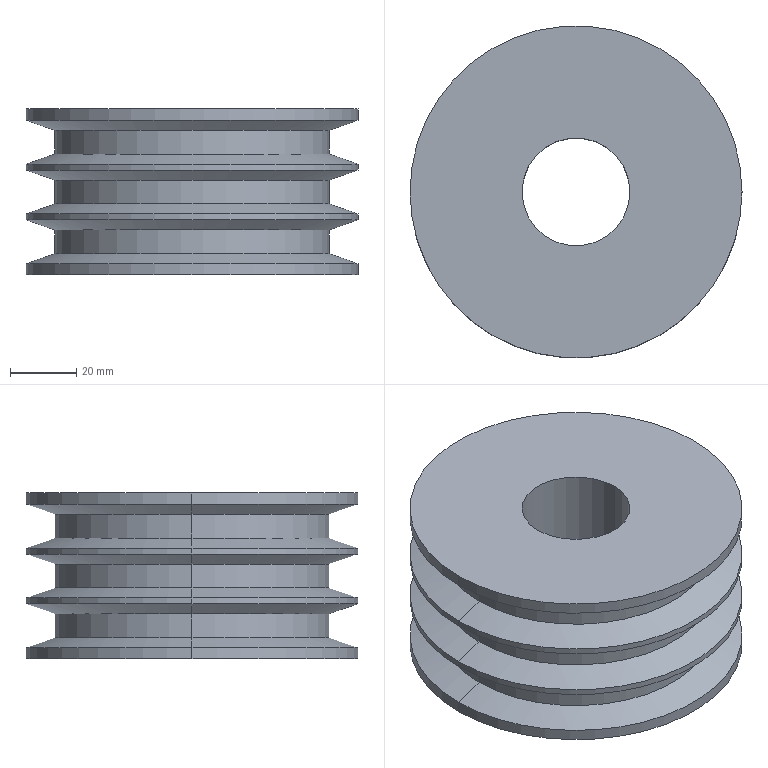Part | SolidWorks | features ICE 6, Extrusion 1, RevCut 1 | 1 solid | 30 faces | box 100 x 100 x 50 mm | volume 274116 mm3 | cylinder 16 | cone 12 | plane 2 | commonest cylinder face diameters 100 x8 82.6 x6 32.5 x2
STEP:
#1=CARTESIAN_POINT('',(41.3,0.,26.396));
#2=VERTEX_POINT('',#1);
#3=CARTESIAN_POINT('',(-41.3,0.,26.396));
#4=VERTEX_POINT('',#3);
#5=CARTESIAN_POINT('',(0.,0.,26.396));
#6=DIRECTION('',(0.,0.,1.));
#7=DIRECTION('',(1.,0.,0.));
#8=AXIS2_PLACEMENT_3D('',#5,#6,#7);
#9=CIRCLE('',#8,41.3);
#10=EDGE_CURVE('',#2,#4,#9,.T.);
#11=ORIENTED_EDGE('',*,*,#10,.F.);
#12=CARTESIAN_POINT('',(50.,0.,23.4));
#13=VERTEX_POINT('',#12);
#14=CARTESIAN_POINT('',(41.3,0.,26.396));
#15=DIRECTION('',(0.9455,0.,-0.3256));
#16=VECTOR('',#15,1000.);
#17=LINE('',#14,#16);
#18=EDGE_CURVE('',#2,#13,#17,.T.);
#19=ORIENTED_EDGE('',*,*,#18,.T.);
#20=CARTESIAN_POINT('',(-50.,0.,23.4));
#21=VERTEX_POINT('',#20);
#22=CARTESIAN_POINT('',(0.,0.,23.4));
#23=DIRECTION('',(0.,0.,1.));
#24=DIRECTION('',(1.,0.,0.));
#25=AXIS2_PLACEMENT_3D('',#22,#23,#24);
#26=CIRCLE('',#25,50.);
#27=EDGE_CURVE('',#13,#21,#26,.T.);
#28=ORIENTED_EDGE('',*,*,#27,.T.);
#29=CARTESIAN_POINT('',(-41.3,0.,26.396));
#30=DIRECTION('',(-0.9455,0.,-0.3256));
#31=VECTOR('',#30,1000.);
#32=LINE('',#29,#31);
#33=EDGE_CURVE('',#4,#21,#32,.T.);
#34=ORIENTED_EDGE('',*,*,#33,.F.);
#35=EDGE_LOOP('',(#11,#19,#28,#34));
#36=FACE_OUTER_BOUND('',#35,.T.);
#37=CARTESIAN_POINT('',(0.,0.,26.396));
#38=DIRECTION('',(0.,0.,-1.));
#39=DIRECTION('',(-1.,0.,0.));
#40=AXIS2_PLACEMENT_3D('',#37,#38,#39);
#41=CONICAL_SURFACE('',#40,41.3,1.239);
#42=ADVANCED_FACE('',(#36),#41,.T.);
#43=ORIENTED_EDGE('',*,*,#10,.T.);
#44=CARTESIAN_POINT('',(-41.3,0.,33.604));
#45=VERTEX_POINT('',#44);
#46=CARTESIAN_POINT('',(-41.3,0.,0.));
#47=DIRECTION('',(0.,0.,1.));
#48=VECTOR('',#47,1000.);
#49=LINE('',#46,#48);
#50=EDGE_CURVE('',#4,#45,#49,.T.);
#51=ORIENTED_EDGE('',*,*,#50,.T.);
#52=CARTESIAN_POINT('',(41.3,0.,33.604));
#53=VERTEX_POINT('',#52);
#54=CARTESIAN_POINT('',(0.,0.,33.604));
#55=DIRECTION('',(0.,0.,1.));
#56=DIRECTION('',(1.,0.,0.));
#57=AXIS2_PLACEMENT_3D('',#54,#55,#56);
#58=CIRCLE('',#57,41.3);
#59=EDGE_CURVE('',#53,#45,#58,.T.);
#60=ORIENTED_EDGE('',*,*,#59,.F.);
#61=CARTESIAN_POINT('',(41.3,0.,0.));
#62=DIRECTION('',(0.,0.,1.));
#63=VECTOR('',#62,1000.);
#64=LINE('',#61,#63);
#65=EDGE_CURVE('',#2,#53,#64,.T.);
#66=ORIENTED_EDGE('',*,*,#65,.F.);
#67=EDGE_LOOP('',(#43,#51,#60,#66));
#68=FACE_OUTER_BOUND('',#67,.T.);
#69=CARTESIAN_POINT('',(0.,0.,0.));
#70=DIRECTION('',(0.,0.,1.));
#71=DIRECTION('',(1.,0.,0.));
#72=AXIS2_PLACEMENT_3D('',#69,#70,#71);
#73=CYLINDRICAL_SURFACE('',#72,41.3);
#74=ADVANCED_FACE('',(#68),#73,.T.);
#75=ORIENTED_EDGE('',*,*,#59,.T.);
#76=CARTESIAN_POINT('',(-50.,0.,36.6));
#77=VERTEX_POINT('',#76);
#78=CARTESIAN_POINT('',(-50.,0.,36.6));
#79=DIRECTION('',(-0.9455,0.,0.3256));
#80=VECTOR('',#79,1000.);
#81=LINE('',#78,#80);
#82=EDGE_CURVE('',#45,#77,#81,.T.);
#83=ORIENTED_EDGE('',*,*,#82,.T.);
#84=CARTESIAN_POINT('',(50.,0.,36.6));
#85=VERTEX_POINT('',#84);
#86=CARTESIAN_POINT('',(0.,0.,36.6));
#87=DIRECTION('',(0.,0.,1.));
#88=DIRECTION('',(1.,0.,0.));
#89=AXIS2_PLACEMENT_3D('',#86,#87,#88);
#90=CIRCLE('',#89,50.);
#91=EDGE_CURVE('',#85,#77,#90,.T.);
#92=ORIENTED_EDGE('',*,*,#91,.F.);
#93=CARTESIAN_POINT('',(50.,0.,36.6));
#94=DIRECTION('',(0.9455,0.,0.3256));
#95=VECTOR('',#94,1000.);
#96=LINE('',#93,#95);
#97=EDGE_CURVE('',#53,#85,#96,.T.);
#98=ORIENTED_EDGE('',*,*,#97,.F.);
#99=EDGE_LOOP('',(#75,#83,#92,#98));
#100=FACE_OUTER_BOUND('',#99,.T.);
#101=CARTESIAN_POINT('',(0.,0.,36.6));
#102=DIRECTION('',(0.,0.,1.));
#103=DIRECTION('',(1.,0.,0.));
#104=AXIS2_PLACEMENT_3D('',#101,#102,#103);
#105=CONICAL_SURFACE('',#104,50.,1.239);
#106=ADVANCED_FACE('',(#100),#105,.T.);
#107=ORIENTED_EDGE('',*,*,#27,.F.);
#108=CARTESIAN_POINT('',(50.,0.,21.6));
#109=VERTEX_POINT('',#108);
#110=CARTESIAN_POINT('',(50.,0.,40.));
#111=DIRECTION('',(0.,0.,-1.));
#112=VECTOR('',#111,1000.);
#113=LINE('',#110,#112);
#114=EDGE_CURVE('',#13,#109,#113,.T.);
#115=ORIENTED_EDGE('',*,*,#114,.T.);
#116=CARTESIAN_POINT('',(-50.,0.,21.6));
#117=VERTEX_POINT('',#116);
#118=CARTESIAN_POINT('',(0.,0.,21.6));
#119=DIRECTION('',(0.,0.,1.));
#120=DIRECTION('',(1.,0.,0.));
#121=AXIS2_PLACEMENT_3D('',#118,#119,#120);
#122=CIRCLE('',#121,50.);
#123=EDGE_CURVE('',#109,#117,#122,.T.);
#124=ORIENTED_EDGE('',*,*,#123,.T.);
#125=CARTESIAN_POINT('',(-50.,0.,40.));
#126=DIRECTION('',(0.,0.,-1.));
#127=VECTOR('',#126,1000.);
#128=LINE('',#125,#127);
#129=EDGE_CURVE('',#21,#117,#128,.T.);
#130=ORIENTED_EDGE('',*,*,#129,.F.);
#131=EDGE_LOOP('',(#107,#115,#124,#130));
#132=FACE_OUTER_BOUND('',#131,.T.);
#133=CARTESIAN_POINT('',(0.,0.,40.));
#134=DIRECTION('',(0.,0.,-1.));
#135=DIRECTION('',(-1.,0.,0.));
#136=AXIS2_PLACEMENT_3D('',#133,#134,#135);
#137=CYLINDRICAL_SURFACE('',#136,50.);
#138=ADVANCED_FACE('',(#132),#137,.T.);
#139=CARTESIAN_POINT('',(41.3,0.,11.396));
#140=VERTEX_POINT('',#139);
#141=CARTESIAN_POINT('',(-41.3,0.,11.396));
#142=VERTEX_POINT('',#141);
#143=CARTESIAN_POINT('',(0.,0.,11.396));
#144=DIRECTION('',(0.,0.,1.));
#145=DIRECTION('',(1.,0.,0.));
#146=AXIS2_PLACEMENT_3D('',#143,#144,#145);
#147=CIRCLE('',#146,41.3);
#148=EDGE_CURVE('',#140,#142,#147,.T.);
#149=ORIENTED_EDGE('',*,*,#148,.F.);
#150=CARTESIAN_POINT('',(50.,0.,8.4));
#151=VERTEX_POINT('',#150);
#152=CARTESIAN_POINT('',(41.3,0.,11.396));
#153=DIRECTION('',(0.9455,0.,-0.3256));
#154=VECTOR('',#153,1000.);
#155=LINE('',#152,#154);
#156=EDGE_CURVE('',#140,#151,#155,.T.);
#157=ORIENTED_EDGE('',*,*,#156,.T.);
#158=CARTESIAN_POINT('',(-50.,0.,8.4));
#159=VERTEX_POINT('',#158);
#160=CARTESIAN_POINT('',(0.,0.,8.4));
#161=DIRECTION('',(0.,0.,1.));
#162=DIRECTION('',(1.,0.,0.));
#163=AXIS2_PLACEMENT_3D('',#160,#161,#162);
#164=CIRCLE('',#163,50.);
#165=EDGE_CURVE('',#151,#159,#164,.T.);
#166=ORIENTED_EDGE('',*,*,#165,.T.);
#167=CARTESIAN_POINT('',(-41.3,0.,11.396));
#168=DIRECTION('',(-0.9455,0.,-0.3256));
#169=VECTOR('',#168,1000.);
#170=LINE('',#167,#169);
#171=EDGE_CURVE('',#142,#159,#170,.T.);
#172=ORIENTED_EDGE('',*,*,#171,.F.);
#173=EDGE_LOOP('',(#149,#157,#166,#172));
#174=FACE_OUTER_BOUND('',#173,.T.);
#175=CARTESIAN_POINT('',(0.,0.,11.396));
#176=DIRECTION('',(0.,0.,-1.));
#177=DIRECTION('',(-1.,0.,0.));
#178=AXIS2_PLACEMENT_3D('',#175,#176,#177);
#179=CONICAL_SURFACE('',#178,41.3,1.239);
#180=ADVANCED_FACE('',(#174),#179,.T.);
#181=ORIENTED_EDGE('',*,*,#148,.T.);
#182=CARTESIAN_POINT('',(-41.3,0.,18.604));
#183=VERTEX_POINT('',#182);
#184=CARTESIAN_POINT('',(-41.3,0.,0.));
#185=DIRECTION('',(0.,0.,1.));
#186=VECTOR('',#185,1000.);
#187=LINE('',#184,#186);
#188=EDGE_CURVE('',#142,#183,#187,.T.);
#189=ORIENTED_EDGE('',*,*,#188,.T.);
#190=CARTESIAN_POINT('',(41.3,0.,18.604));
#191=VERTEX_POINT('',#190);
#192=CARTESIAN_POINT('',(0.,0.,18.604));
#193=DIRECTION('',(0.,0.,1.));
#194=DIRECTION('',(1.,0.,0.));
#195=AXIS2_PLACEMENT_3D('',#192,#193,#194);
#196=CIRCLE('',#195,41.3);
#197=EDGE_CURVE('',#191,#183,#196,.T.);
#198=ORIENTED_EDGE('',*,*,#197,.F.);
#199=CARTESIAN_POINT('',(41.3,0.,0.));
#200=DIRECTION('',(0.,0.,1.));
#201=VECTOR('',#200,1000.);
#202=LINE('',#199,#201);
#203=EDGE_CURVE('',#140,#191,#202,.T.);
#204=ORIENTED_EDGE('',*,*,#203,.F.);
#205=EDGE_LOOP('',(#181,#189,#198,#204));
#206=FACE_OUTER_BOUND('',#205,.T.);
#207=CARTESIAN_POINT('',(0.,0.,0.));
#208=DIRECTION('',(0.,0.,1.));
#209=DIRECTION('',(1.,0.,0.));
#210=AXIS2_PLACEMENT_3D('',#207,#208,#209);
#211=CYLINDRICAL_SURFACE('',#210,41.3);
#212=ADVANCED_FACE('',(#206),#211,.T.);
#213=ORIENTED_EDGE('',*,*,#197,.T.);
#214=CARTESIAN_POINT('',(-50.,0.,21.6));
#215=DIRECTION('',(-0.9455,0.,0.3256));
#216=VECTOR('',#215,1000.);
#217=LINE('',#214,#216);
#218=EDGE_CURVE('',#183,#117,#217,.T.);
#219=ORIENTED_EDGE('',*,*,#218,.T.);
#220=ORIENTED_EDGE('',*,*,#123,.F.);
#221=CARTESIAN_POINT('',(50.,0.,21.6));
#222=DIRECTION('',(0.9455,0.,0.3256));
#223=VECTOR('',#222,1000.);
#224=LINE('',#221,#223);
#225=EDGE_CURVE('',#191,#109,#224,.T.);
#226=ORIENTED_EDGE('',*,*,#225,.F.);
#227=EDGE_LOOP('',(#213,#219,#220,#226));
#228=FACE_OUTER_BOUND('',#227,.T.);
#229=CARTESIAN_POINT('',(0.,0.,21.6));
#230=DIRECTION('',(0.,0.,1.));
#231=DIRECTION('',(1.,0.,0.));
#232=AXIS2_PLACEMENT_3D('',#229,#230,#231);
#233=CONICAL_SURFACE('',#232,50.,1.239);
#234=ADVANCED_FACE('',(#228),#233,.T.);
#235=ORIENTED_EDGE('',*,*,#165,.F.);
#236=CARTESIAN_POINT('',(50.,0.,6.6));
#237=VERTEX_POINT('',#236);
#238=CARTESIAN_POINT('',(50.,0.,40.));
#239=DIRECTION('',(0.,0.,-1.));
#240=VECTOR('',#239,1000.);
#241=LINE('',#238,#240);
#242=EDGE_CURVE('',#151,#237,#241,.T.);
#243=ORIENTED_EDGE('',*,*,#242,.T.);
#244=CARTESIAN_POINT('',(-50.,0.,6.6));
#245=VERTEX_POINT('',#244);
#246=CARTESIAN_POINT('',(0.,0.,6.6));
#247=DIRECTION('',(0.,0.,1.));
#248=DIRECTION('',(1.,0.,0.));
#249=AXIS2_PLACEMENT_3D('',#246,#247,#248);
#250=CIRCLE('',#249,50.);
#251=EDGE_CURVE('',#237,#245,#250,.T.);
#252=ORIENTED_EDGE('',*,*,#251,.T.);
#253=CARTESIAN_POINT('',(-50.,0.,40.));
#254=DIRECTION('',(0.,0.,-1.));
#255=VECTOR('',#254,1000.);
#256=LINE('',#253,#255);
#257=EDGE_CURVE('',#159,#245,#256,.T.);
#258=ORIENTED_EDGE('',*,*,#257,.F.);
#259=EDGE_LOOP('',(#235,#243,#252,#258));
#260=FACE_OUTER_BOUND('',#259,.T.);
#261=CARTESIAN_POINT('',(0.,0.,40.));
#262=DIRECTION('',(0.,0.,-1.));
#263=DIRECTION('',(-1.,0.,0.));
#264=AXIS2_PLACEMENT_3D('',#261,#262,#263);
#265=CYLINDRICAL_SURFACE('',#264,50.);
#266=ADVANCED_FACE('',(#260),#265,.T.);
#267=CARTESIAN_POINT('',(41.3,0.,-3.604));
#268=VERTEX_POINT('',#267);
#269=CARTESIAN_POINT('',(-41.3,0.,-3.604));
#270=VERTEX_POINT('',#269);
#271=CARTESIAN_POINT('',(0.,0.,-3.604));
#272=DIRECTION('',(0.,0.,1.));
#273=DIRECTION('',(1.,0.,0.));
#274=AXIS2_PLACEMENT_3D('',#271,#272,#273);
#275=CIRCLE('',#274,41.3);
#276=EDGE_CURVE('',#268,#270,#275,.T.);
#277=ORIENTED_EDGE('',*,*,#276,.F.);
#278=CARTESIAN_POINT('',(50.,0.,-6.6));
#279=VERTEX_POINT('',#278);
#280=CARTESIAN_POINT('',(41.3,0.,-3.604));
#281=DIRECTION('',(0.9455,0.,-0.3256));
#282=VECTOR('',#281,1000.);
#283=LINE('',#280,#282);
#284=EDGE_CURVE('',#268,#279,#283,.T.);
#285=ORIENTED_EDGE('',*,*,#284,.T.);
#286=CARTESIAN_POINT('',(-50.,0.,-6.6));
#287=VERTEX_POINT('',#286);
#288=CARTESIAN_POINT('',(0.,0.,-6.6));
#289=DIRECTION('',(0.,0.,1.));
#290=DIRECTION('',(1.,0.,0.));
#291=AXIS2_PLACEMENT_3D('',#288,#289,#290);
#292=CIRCLE('',#291,50.);
#293=EDGE_CURVE('',#279,#287,#292,.T.);
#294=ORIENTED_EDGE('',*,*,#293,.T.);
#295=CARTESIAN_POINT('',(-41.3,0.,-3.604));
#296=DIRECTION('',(-0.9455,0.,-0.3256));
#297=VECTOR('',#296,1000.);
#298=LINE('',#295,#297);
#299=EDGE_CURVE('',#270,#287,#298,.T.);
#300=ORIENTED_EDGE('',*,*,#299,.F.);
#301=EDGE_LOOP('',(#277,#285,#294,#300));
#302=FACE_OUTER_BOUND('',#301,.T.);
#303=CARTESIAN_POINT('',(0.,0.,-3.604));
#304=DIRECTION('',(0.,0.,-1.));
#305=DIRECTION('',(-1.,0.,0.));
#306=AXIS2_PLACEMENT_3D('',#303,#304,#305);
#307=CONICAL_SURFACE('',#306,41.3,1.239);
#308=ADVANCED_FACE('',(#302),#307,.T.);
#309=ORIENTED_EDGE('',*,*,#276,.T.);
#310=CARTESIAN_POINT('',(-41.3,0.,3.604));
#311=VERTEX_POINT('',#310);
#312=CARTESIAN_POINT('',(-41.3,0.,0.));
#313=DIRECTION('',(0.,0.,1.));
#314=VECTOR('',#313,1000.);
#315=LINE('',#312,#314);
#316=EDGE_CURVE('',#270,#311,#315,.T.);
#317=ORIENTED_EDGE('',*,*,#316,.T.);
#318=CARTESIAN_POINT('',(41.3,0.,3.604));
#319=VERTEX_POINT('',#318);
#320=CARTESIAN_POINT('',(0.,0.,3.604));
#321=DIRECTION('',(0.,0.,1.));
#322=DIRECTION('',(1.,0.,0.));
#323=AXIS2_PLACEMENT_3D('',#320,#321,#322);
#324=CIRCLE('',#323,41.3);
#325=EDGE_CURVE('',#319,#311,#324,.T.);
#326=ORIENTED_EDGE('',*,*,#325,.F.);
#327=CARTESIAN_POINT('',(41.3,0.,0.));
#328=DIRECTION('',(0.,0.,1.));
#329=VECTOR('',#328,1000.);
#330=LINE('',#327,#329);
#331=EDGE_CURVE('',#268,#319,#330,.T.);
#332=ORIENTED_EDGE('',*,*,#331,.F.);
#333=EDGE_LOOP('',(#309,#317,#326,#332));
#334=FACE_OUTER_BOUND('',#333,.T.);
#335=CARTESIAN_POINT('',(0.,0.,0.));
#336=DIRECTION('',(0.,0.,1.));
#337=DIRECTION('',(1.,0.,0.));
#338=AXIS2_PLACEMENT_3D('',#335,#336,#337);
#339=CYLINDRICAL_SURFACE('',#338,41.3);
#340=ADVANCED_FACE('',(#334),#339,.T.);
#341=ORIENTED_EDGE('',*,*,#325,.T.);
#342=CARTESIAN_POINT('',(-50.,0.,6.6));
#343=DIRECTION('',(-0.9455,0.,0.3256));
#344=VECTOR('',#343,1000.);
#345=LINE('',#342,#344);
#346=EDGE_CURVE('',#311,#245,#345,.T.);
#347=ORIENTED_EDGE('',*,*,#346,.T.);
#348=ORIENTED_EDGE('',*,*,#251,.F.);
#349=CARTESIAN_POINT('',(50.,0.,6.6));
#350=DIRECTION('',(0.9455,0.,0.3256));
#351=VECTOR('',#350,1000.);
#352=LINE('',#349,#351);
#353=EDGE_CURVE('',#319,#237,#352,.T.);
#354=ORIENTED_EDGE('',*,*,#353,.F.);
#355=EDGE_LOOP('',(#341,#347,#348,#354));
#356=FACE_OUTER_BOUND('',#355,.T.);
#357=CARTESIAN_POINT('',(0.,0.,6.6));
#358=DIRECTION('',(0.,0.,1.));
#359=DIRECTION('',(1.,0.,0.));
#360=AXIS2_PLACEMENT_3D('',#357,#358,#359);
#361=CONICAL_SURFACE('',#360,50.,1.239);
#362=ADVANCED_FACE('',(#356),#361,.T.);
#363=CARTESIAN_POINT('',(50.,0.,40.));
#364=VERTEX_POINT('',#363);
#365=CARTESIAN_POINT('',(-50.,0.,40.));
#366=VERTEX_POINT('',#365);
#367=CARTESIAN_POINT('',(0.,0.,40.));
#368=DIRECTION('',(0.,0.,1.));
#369=DIRECTION('',(1.,0.,0.));
#370=AXIS2_PLACEMENT_3D('',#367,#368,#369);
#371=CIRCLE('',#370,50.);
#372=EDGE_CURVE('',#364,#366,#371,.T.);
#373=ORIENTED_EDGE('',*,*,#372,.F.);
#374=CARTESIAN_POINT('',(50.,0.,40.));
#375=DIRECTION('',(0.,0.,-1.));
#376=VECTOR('',#375,1000.);
#377=LINE('',#374,#376);
#378=EDGE_CURVE('',#364,#85,#377,.T.);
#379=ORIENTED_EDGE('',*,*,#378,.T.);
#380=ORIENTED_EDGE('',*,*,#91,.T.);
#381=CARTESIAN_POINT('',(-50.,0.,40.));
#382=DIRECTION('',(0.,0.,-1.));
#383=VECTOR('',#382,1000.);
#384=LINE('',#381,#383);
#385=EDGE_CURVE('',#366,#77,#384,.T.);
#386=ORIENTED_EDGE('',*,*,#385,.F.);
#387=EDGE_LOOP('',(#373,#379,#380,#386));
#388=FACE_OUTER_BOUND('',#387,.T.);
#389=CARTESIAN_POINT('',(0.,0.,40.));
#390=DIRECTION('',(0.,0.,-1.));
#391=DIRECTION('',(-1.,0.,0.));
#392=AXIS2_PLACEMENT_3D('',#389,#390,#391);
#393=CYLINDRICAL_SURFACE('',#392,50.);
#394=ADVANCED_FACE('',(#388),#393,.T.);
#395=CARTESIAN_POINT('',(-16.25,0.,-10.));
#396=VERTEX_POINT('',#395);
#397=CARTESIAN_POINT('',(16.25,0.,-10.));
#398=VERTEX_POINT('',#397);
#399=CARTESIAN_POINT('',(0.,0.,-10.));
#400=DIRECTION('',(0.,0.,1.));
#401=DIRECTION('',(-1.,0.,0.));
#402=AXIS2_PLACEMENT_3D('',#399,#400,#401);
#403=CIRCLE('',#402,16.25);
#404=EDGE_CURVE('',#396,#398,#403,.T.);
#405=ORIENTED_EDGE('',*,*,#404,.F.);
#406=CARTESIAN_POINT('',(-16.25,0.,40.));
#407=VERTEX_POINT('',#406);
#408=CARTESIAN_POINT('',(-16.25,0.,-110.));
#409=DIRECTION('',(0.,0.,1.));
#410=VECTOR('',#409,1000.);
#411=LINE('',#408,#410);
#412=EDGE_CURVE('',#396,#407,#411,.T.);
#413=ORIENTED_EDGE('',*,*,#412,.T.);
#414=CARTESIAN_POINT('',(16.25,0.,40.));
#415=VERTEX_POINT('',#414);
#416=CARTESIAN_POINT('',(0.,0.,40.));
#417=DIRECTION('',(0.,0.,1.));
#418=DIRECTION('',(1.,0.,0.));
#419=AXIS2_PLACEMENT_3D('',#416,#417,#418);
#420=CIRCLE('',#419,16.25);
#421=EDGE_CURVE('',#407,#415,#420,.T.);
#422=ORIENTED_EDGE('',*,*,#421,.T.);
#423=CARTESIAN_POINT('',(16.25,0.,-110.));
#424=DIRECTION('',(0.,0.,1.));
#425=VECTOR('',#424,1000.);
#426=LINE('',#423,#425);
#427=EDGE_CURVE('',#398,#415,#426,.T.);
#428=ORIENTED_EDGE('',*,*,#427,.F.);
#429=EDGE_LOOP('',(#405,#413,#422,#428));
#430=FACE_OUTER_BOUND('',#429,.T.);
#431=CARTESIAN_POINT('',(0.,0.,-110.));
#432=DIRECTION('',(0.,0.,1.));
#433=DIRECTION('',(1.,0.,0.));
#434=AXIS2_PLACEMENT_3D('',#431,#432,#433);
#435=CYLINDRICAL_SURFACE('',#434,16.25);
#436=ADVANCED_FACE('',(#430),#435,.F.);
#437=ORIENTED_EDGE('',*,*,#293,.F.);
#438=CARTESIAN_POINT('',(50.,0.,-10.));
#439=VERTEX_POINT('',#438);
#440=CARTESIAN_POINT('',(50.,0.,40.));
#441=DIRECTION('',(0.,0.,-1.));
#442=VECTOR('',#441,1000.);
#443=LINE('',#440,#442);
#444=EDGE_CURVE('',#279,#439,#443,.T.);
#445=ORIENTED_EDGE('',*,*,#444,.T.);
#446=CARTESIAN_POINT('',(-50.,0.,-10.));
#447=VERTEX_POINT('',#446);
#448=CARTESIAN_POINT('',(0.,0.,-10.));
#449=DIRECTION('',(0.,0.,-1.));
#450=DIRECTION('',(-1.,0.,0.));
#451=AXIS2_PLACEMENT_3D('',#448,#449,#450);
#452=CIRCLE('',#451,50.);
#453=EDGE_CURVE('',#447,#439,#452,.T.);
#454=ORIENTED_EDGE('',*,*,#453,.F.);
#455=CARTESIAN_POINT('',(-50.,0.,40.));
#456=DIRECTION('',(0.,0.,-1.));
#457=VECTOR('',#456,1000.);
#458=LINE('',#455,#457);
#459=EDGE_CURVE('',#287,#447,#458,.T.);
#460=ORIENTED_EDGE('',*,*,#459,.F.);
#461=EDGE_LOOP('',(#437,#445,#454,#460));
#462=FACE_OUTER_BOUND('',#461,.T.);
#463=CARTESIAN_POINT('',(0.,0.,40.));
#464=DIRECTION('',(0.,0.,-1.));
#465=DIRECTION('',(-1.,0.,0.));
#466=AXIS2_PLACEMENT_3D('',#463,#464,#465);
#467=CYLINDRICAL_SURFACE('',#466,50.);
#468=ADVANCED_FACE('',(#462),#467,.T.);
#469=ORIENTED_EDGE('',*,*,#444,.F.);
#470=CARTESIAN_POINT('',(0.,0.,-6.6));
#471=DIRECTION('',(0.,0.,1.));
#472=DIRECTION('',(1.,0.,0.));
#473=AXIS2_PLACEMENT_3D('',#470,#471,#472);
#474=CIRCLE('',#473,50.);
#475=EDGE_CURVE('',#287,#279,#474,.T.);
#476=ORIENTED_EDGE('',*,*,#475,.F.);
#477=ORIENTED_EDGE('',*,*,#459,.T.);
#478=CARTESIAN_POINT('',(0.,0.,-10.));
#479=DIRECTION('',(0.,0.,-1.));
#480=DIRECTION('',(-1.,0.,0.));
#481=AXIS2_PLACEMENT_3D('',#478,#479,#480);
#482=CIRCLE('',#481,50.);
#483=EDGE_CURVE('',#439,#447,#482,.T.);
#484=ORIENTED_EDGE('',*,*,#483,.F.);
#485=EDGE_LOOP('',(#469,#476,#477,#484));
#486=FACE_OUTER_BOUND('',#485,.T.);
#487=CARTESIAN_POINT('',(0.,0.,40.));
#488=DIRECTION('',(0.,0.,-1.));
#489=DIRECTION('',(-1.,0.,0.));
#490=AXIS2_PLACEMENT_3D('',#487,#488,#489);
#491=CYLINDRICAL_SURFACE('',#490,50.);
#492=ADVANCED_FACE('',(#486),#491,.T.);
#493=ORIENTED_EDGE('',*,*,#412,.F.);
#494=CARTESIAN_POINT('',(0.,0.,-10.));
#495=DIRECTION('',(0.,0.,1.));
#496=DIRECTION('',(-1.,0.,0.));
#497=AXIS2_PLACEMENT_3D('',#494,#495,#496);
#498=CIRCLE('',#497,16.25);
#499=EDGE_CURVE('',#398,#396,#498,.T.);
#500=ORIENTED_EDGE('',*,*,#499,.F.);
#501=ORIENTED_EDGE('',*,*,#427,.T.);
#502=CARTESIAN_POINT('',(0.,0.,40.));
#503=DIRECTION('',(0.,0.,1.));
#504=DIRECTION('',(1.,0.,0.));
#505=AXIS2_PLACEMENT_3D('',#502,#503,#504);
#506=CIRCLE('',#505,16.25);
#507=EDGE_CURVE('',#415,#407,#506,.T.);
#508=ORIENTED_EDGE('',*,*,#507,.T.);
#509=EDGE_LOOP('',(#493,#500,#501,#508));
#510=FACE_OUTER_BOUND('',#509,.T.);
#511=CARTESIAN_POINT('',(0.,0.,-110.));
#512=DIRECTION('',(0.,0.,1.));
#513=DIRECTION('',(1.,0.,0.));
#514=AXIS2_PLACEMENT_3D('',#511,#512,#513);
#515=CYLINDRICAL_SURFACE('',#514,16.25);
#516=ADVANCED_FACE('',(#510),#515,.F.);
#517=ORIENTED_EDGE('',*,*,#378,.F.);
#518=CARTESIAN_POINT('',(0.,0.,40.));
#519=DIRECTION('',(0.,0.,1.));
#520=DIRECTION('',(1.,0.,0.));
#521=AXIS2_PLACEMENT_3D('',#518,#519,#520);
#522=CIRCLE('',#521,50.);
#523=EDGE_CURVE('',#366,#364,#522,.T.);
#524=ORIENTED_EDGE('',*,*,#523,.F.);
#525=ORIENTED_EDGE('',*,*,#385,.T.);
#526=CARTESIAN_POINT('',(0.,0.,36.6));
#527=DIRECTION('',(0.,0.,1.));
#528=DIRECTION('',(1.,0.,0.));
#529=AXIS2_PLACEMENT_3D('',#526,#527,#528);
#530=CIRCLE('',#529,50.);
#531=EDGE_CURVE('',#77,#85,#530,.T.);
#532=ORIENTED_EDGE('',*,*,#531,.T.);
#533=EDGE_LOOP('',(#517,#524,#525,#532));
#534=FACE_OUTER_BOUND('',#533,.T.);
#535=CARTESIAN_POINT('',(0.,0.,40.));
#536=DIRECTION('',(0.,0.,-1.));
#537=DIRECTION('',(-1.,0.,0.));
#538=AXIS2_PLACEMENT_3D('',#535,#536,#537);
#539=CYLINDRICAL_SURFACE('',#538,50.);
#540=ADVANCED_FACE('',(#534),#539,.T.);
#541=ORIENTED_EDGE('',*,*,#507,.F.);
#542=ORIENTED_EDGE('',*,*,#421,.F.);
#543=EDGE_LOOP('',(#541,#542));
#544=FACE_BOUND('',#543,.T.);
#545=ORIENTED_EDGE('',*,*,#523,.T.);
#546=ORIENTED_EDGE('',*,*,#372,.T.);
#547=EDGE_LOOP('',(#545,#546));
#548=FACE_OUTER_BOUND('',#547,.T.);
#549=CARTESIAN_POINT('',(0.,0.,40.));
#550=DIRECTION('',(0.,0.,1.));
#551=DIRECTION('',(1.,0.,0.));
#552=AXIS2_PLACEMENT_3D('',#549,#550,#551);
#553=PLANE('',#552);
#554=ADVANCED_FACE('',(#544,#548),#553,.T.);
#555=ORIENTED_EDGE('',*,*,#346,.F.);
#556=CARTESIAN_POINT('',(0.,0.,3.604));
#557=DIRECTION('',(0.,0.,1.));
#558=DIRECTION('',(1.,0.,0.));
#559=AXIS2_PLACEMENT_3D('',#556,#557,#558);
#560=CIRCLE('',#559,41.3);
#561=EDGE_CURVE('',#311,#319,#560,.T.);
#562=ORIENTED_EDGE('',*,*,#561,.T.);
#563=ORIENTED_EDGE('',*,*,#353,.T.);
#564=CARTESIAN_POINT('',(0.,0.,6.6));
#565=DIRECTION('',(0.,0.,1.));
#566=DIRECTION('',(1.,0.,0.));
#567=AXIS2_PLACEMENT_3D('',#564,#565,#566);
#568=CIRCLE('',#567,50.);
#569=EDGE_CURVE('',#245,#237,#568,.T.);
#570=ORIENTED_EDGE('',*,*,#569,.F.);
#571=EDGE_LOOP('',(#555,#562,#563,#570));
#572=FACE_OUTER_BOUND('',#571,.T.);
#573=CARTESIAN_POINT('',(0.,0.,6.6));
#574=DIRECTION('',(0.,0.,1.));
#575=DIRECTION('',(1.,0.,0.));
#576=AXIS2_PLACEMENT_3D('',#573,#574,#575);
#577=CONICAL_SURFACE('',#576,50.,1.239);
#578=ADVANCED_FACE('',(#572),#577,.T.);
#579=ORIENTED_EDGE('',*,*,#316,.F.);
#580=CARTESIAN_POINT('',(0.,0.,-3.604));
#581=DIRECTION('',(0.,0.,1.));
#582=DIRECTION('',(1.,0.,0.));
#583=AXIS2_PLACEMENT_3D('',#580,#581,#582);
#584=CIRCLE('',#583,41.3);
#585=EDGE_CURVE('',#270,#268,#584,.T.);
#586=ORIENTED_EDGE('',*,*,#585,.T.);
#587=ORIENTED_EDGE('',*,*,#331,.T.);
#588=ORIENTED_EDGE('',*,*,#561,.F.);
#589=EDGE_LOOP('',(#579,#586,#587,#588));
#590=FACE_OUTER_BOUND('',#589,.T.);
#591=CARTESIAN_POINT('',(0.,0.,0.));
#592=DIRECTION('',(0.,0.,1.));
#593=DIRECTION('',(1.,0.,0.));
#594=AXIS2_PLACEMENT_3D('',#591,#592,#593);
#595=CYLINDRICAL_SURFACE('',#594,41.3);
#596=ADVANCED_FACE('',(#590),#595,.T.);
#597=ORIENTED_EDGE('',*,*,#284,.F.);
#598=ORIENTED_EDGE('',*,*,#585,.F.);
#599=ORIENTED_EDGE('',*,*,#299,.T.);
#600=ORIENTED_EDGE('',*,*,#475,.T.);
#601=EDGE_LOOP('',(#597,#598,#599,#600));
#602=FACE_OUTER_BOUND('',#601,.T.);
#603=CARTESIAN_POINT('',(0.,0.,-3.604));
#604=DIRECTION('',(0.,0.,-1.));
#605=DIRECTION('',(-1.,0.,0.));
#606=AXIS2_PLACEMENT_3D('',#603,#604,#605);
#607=CONICAL_SURFACE('',#606,41.3,1.239);
#608=ADVANCED_FACE('',(#602),#607,.T.);
#609=ORIENTED_EDGE('',*,*,#242,.F.);
#610=CARTESIAN_POINT('',(0.,0.,8.4));
#611=DIRECTION('',(0.,0.,1.));
#612=DIRECTION('',(1.,0.,0.));
#613=AXIS2_PLACEMENT_3D('',#610,#611,#612);
#614=CIRCLE('',#613,50.);
#615=EDGE_CURVE('',#159,#151,#614,.T.);
#616=ORIENTED_EDGE('',*,*,#615,.F.);
#617=ORIENTED_EDGE('',*,*,#257,.T.);
#618=ORIENTED_EDGE('',*,*,#569,.T.);
#619=EDGE_LOOP('',(#609,#616,#617,#618));
#620=FACE_OUTER_BOUND('',#619,.T.);
#621=CARTESIAN_POINT('',(0.,0.,40.));
#622=DIRECTION('',(0.,0.,-1.));
#623=DIRECTION('',(-1.,0.,0.));
#624=AXIS2_PLACEMENT_3D('',#621,#622,#623);
#625=CYLINDRICAL_SURFACE('',#624,50.);
#626=ADVANCED_FACE('',(#620),#625,.T.);
#627=ORIENTED_EDGE('',*,*,#218,.F.);
#628=CARTESIAN_POINT('',(0.,0.,18.604));
#629=DIRECTION('',(0.,0.,1.));
#630=DIRECTION('',(1.,0.,0.));
#631=AXIS2_PLACEMENT_3D('',#628,#629,#630);
#632=CIRCLE('',#631,41.3);
#633=EDGE_CURVE('',#183,#191,#632,.T.);
#634=ORIENTED_EDGE('',*,*,#633,.T.);
#635=ORIENTED_EDGE('',*,*,#225,.T.);
#636=CARTESIAN_POINT('',(0.,0.,21.6));
#637=DIRECTION('',(0.,0.,1.));
#638=DIRECTION('',(1.,0.,0.));
#639=AXIS2_PLACEMENT_3D('',#636,#637,#638);
#640=CIRCLE('',#639,50.);
#641=EDGE_CURVE('',#117,#109,#640,.T.);
#642=ORIENTED_EDGE('',*,*,#641,.F.);
#643=EDGE_LOOP('',(#627,#634,#635,#642));
#644=FACE_OUTER_BOUND('',#643,.T.);
#645=CARTESIAN_POINT('',(0.,0.,21.6));
#646=DIRECTION('',(0.,0.,1.));
#647=DIRECTION('',(1.,0.,0.));
#648=AXIS2_PLACEMENT_3D('',#645,#646,#647);
#649=CONICAL_SURFACE('',#648,50.,1.239);
#650=ADVANCED_FACE('',(#644),#649,.T.);
#651=ORIENTED_EDGE('',*,*,#188,.F.);
#652=CARTESIAN_POINT('',(0.,0.,11.396));
#653=DIRECTION('',(0.,0.,1.));
#654=DIRECTION('',(1.,0.,0.));
#655=AXIS2_PLACEMENT_3D('',#652,#653,#654);
#656=CIRCLE('',#655,41.3);
#657=EDGE_CURVE('',#142,#140,#656,.T.);
#658=ORIENTED_EDGE('',*,*,#657,.T.);
#659=ORIENTED_EDGE('',*,*,#203,.T.);
#660=ORIENTED_EDGE('',*,*,#633,.F.);
#661=EDGE_LOOP('',(#651,#658,#659,#660));
#662=FACE_OUTER_BOUND('',#661,.T.);
#663=CARTESIAN_POINT('',(0.,0.,0.));
#664=DIRECTION('',(0.,0.,1.));
#665=DIRECTION('',(1.,0.,0.));
#666=AXIS2_PLACEMENT_3D('',#663,#664,#665);
#667=CYLINDRICAL_SURFACE('',#666,41.3);
#668=ADVANCED_FACE('',(#662),#667,.T.);
#669=ORIENTED_EDGE('',*,*,#156,.F.);
#670=ORIENTED_EDGE('',*,*,#657,.F.);
#671=ORIENTED_EDGE('',*,*,#171,.T.);
#672=ORIENTED_EDGE('',*,*,#615,.T.);
#673=EDGE_LOOP('',(#669,#670,#671,#672));
#674=FACE_OUTER_BOUND('',#673,.T.);
#675=CARTESIAN_POINT('',(0.,0.,11.396));
#676=DIRECTION('',(0.,0.,-1.));
#677=DIRECTION('',(-1.,0.,0.));
#678=AXIS2_PLACEMENT_3D('',#675,#676,#677);
#679=CONICAL_SURFACE('',#678,41.3,1.239);
#680=ADVANCED_FACE('',(#674),#679,.T.);
#681=ORIENTED_EDGE('',*,*,#114,.F.);
#682=CARTESIAN_POINT('',(0.,0.,23.4));
#683=DIRECTION('',(0.,0.,1.));
#684=DIRECTION('',(1.,0.,0.));
#685=AXIS2_PLACEMENT_3D('',#682,#683,#684);
#686=CIRCLE('',#685,50.);
#687=EDGE_CURVE('',#21,#13,#686,.T.);
#688=ORIENTED_EDGE('',*,*,#687,.F.);
#689=ORIENTED_EDGE('',*,*,#129,.T.);
#690=ORIENTED_EDGE('',*,*,#641,.T.);
#691=EDGE_LOOP('',(#681,#688,#689,#690));
#692=FACE_OUTER_BOUND('',#691,.T.);
#693=CARTESIAN_POINT('',(0.,0.,40.));
#694=DIRECTION('',(0.,0.,-1.));
#695=DIRECTION('',(-1.,0.,0.));
#696=AXIS2_PLACEMENT_3D('',#693,#694,#695);
#697=CYLINDRICAL_SURFACE('',#696,50.);
#698=ADVANCED_FACE('',(#692),#697,.T.);
#699=ORIENTED_EDGE('',*,*,#82,.F.);
#700=CARTESIAN_POINT('',(0.,0.,33.604));
#701=DIRECTION('',(0.,0.,1.));
#702=DIRECTION('',(1.,0.,0.));
#703=AXIS2_PLACEMENT_3D('',#700,#701,#702);
#704=CIRCLE('',#703,41.3);
#705=EDGE_CURVE('',#45,#53,#704,.T.);
#706=ORIENTED_EDGE('',*,*,#705,.T.);
#707=ORIENTED_EDGE('',*,*,#97,.T.);
#708=ORIENTED_EDGE('',*,*,#531,.F.);
#709=EDGE_LOOP('',(#699,#706,#707,#708));
#710=FACE_OUTER_BOUND('',#709,.T.);
#711=CARTESIAN_POINT('',(0.,0.,36.6));
#712=DIRECTION('',(0.,0.,1.));
#713=DIRECTION('',(1.,0.,0.));
#714=AXIS2_PLACEMENT_3D('',#711,#712,#713);
#715=CONICAL_SURFACE('',#714,50.,1.239);
#716=ADVANCED_FACE('',(#710),#715,.T.);
#717=ORIENTED_EDGE('',*,*,#50,.F.);
#718=CARTESIAN_POINT('',(0.,0.,26.396));
#719=DIRECTION('',(0.,0.,1.));
#720=DIRECTION('',(1.,0.,0.));
#721=AXIS2_PLACEMENT_3D('',#718,#719,#720);
#722=CIRCLE('',#721,41.3);
#723=EDGE_CURVE('',#4,#2,#722,.T.);
#724=ORIENTED_EDGE('',*,*,#723,.T.);
#725=ORIENTED_EDGE('',*,*,#65,.T.);
#726=ORIENTED_EDGE('',*,*,#705,.F.);
#727=EDGE_LOOP('',(#717,#724,#725,#726));
#728=FACE_OUTER_BOUND('',#727,.T.);
#729=CARTESIAN_POINT('',(0.,0.,0.));
#730=DIRECTION('',(0.,0.,1.));
#731=DIRECTION('',(1.,0.,0.));
#732=AXIS2_PLACEMENT_3D('',#729,#730,#731);
#733=CYLINDRICAL_SURFACE('',#732,41.3);
#734=ADVANCED_FACE('',(#728),#733,.T.);
#735=ORIENTED_EDGE('',*,*,#18,.F.);
#736=ORIENTED_EDGE('',*,*,#723,.F.);
#737=ORIENTED_EDGE('',*,*,#33,.T.);
#738=ORIENTED_EDGE('',*,*,#687,.T.);
#739=EDGE_LOOP('',(#735,#736,#737,#738));
#740=FACE_OUTER_BOUND('',#739,.T.);
#741=CARTESIAN_POINT('',(0.,0.,26.396));
#742=DIRECTION('',(0.,0.,-1.));
#743=DIRECTION('',(-1.,0.,0.));
#744=AXIS2_PLACEMENT_3D('',#741,#742,#743);
#745=CONICAL_SURFACE('',#744,41.3,1.239);
#746=ADVANCED_FACE('',(#740),#745,.T.);
#747=ORIENTED_EDGE('',*,*,#499,.T.);
#748=ORIENTED_EDGE('',*,*,#404,.T.);
#749=EDGE_LOOP('',(#747,#748));
#750=FACE_BOUND('',#749,.T.);
#751=ORIENTED_EDGE('',*,*,#453,.T.);
#752=ORIENTED_EDGE('',*,*,#483,.T.);
#753=EDGE_LOOP('',(#751,#752));
#754=FACE_OUTER_BOUND('',#753,.T.);
#755=CARTESIAN_POINT('',(0.,0.,-10.));
#756=DIRECTION('',(0.,0.,-1.));
#757=DIRECTION('',(-1.,0.,0.));
#758=AXIS2_PLACEMENT_3D('',#755,#756,#757);
#759=PLANE('',#758);
#760=ADVANCED_FACE('',(#750,#754),#759,.T.);
#761=CLOSED_SHELL('',(#42,#74,#106,#138,#180,#212,#234,#266,#308,#340,#362,#394,#436,#468,#492,#516,#540,#554,#578,#596,#608,#626,#650,#668,#680,#698,#716,#734,#746,#760));
#762=MANIFOLD_SOLID_BREP('',#761);
#763=CARTESIAN_POINT('',(0.,0.,0.));
#764=DIRECTION('',(0.,0.,1.));
#765=DIRECTION('',(1.,0.,0.));
#766=AXIS2_PLACEMENT_3D('',#763,#764,#765);
#767=(LENGTH_UNIT()NAMED_UNIT(*)SI_UNIT(.MILLI.,.METRE.));
#768=UNCERTAINTY_MEASURE_WITH_UNIT(LENGTH_MEASURE(0.00001),#767,'','');
#769=(NAMED_UNIT(*)PLANE_ANGLE_UNIT()SI_UNIT($,.RADIAN.));
#770=(NAMED_UNIT(*)SI_UNIT($,.STERADIAN.)SOLID_ANGLE_UNIT());
#771=(GEOMETRIC_REPRESENTATION_CONTEXT(3)GLOBAL_UNCERTAINTY_ASSIGNED_CONTEXT((#768))GLOBAL_UNIT_ASSIGNED_CONTEXT((#767,#769,#770))REPRESENTATION_CONTEXT('',''));
#772=ADVANCED_BREP_SHAPE_REPRESENTATION('',(#762,#766),#771);